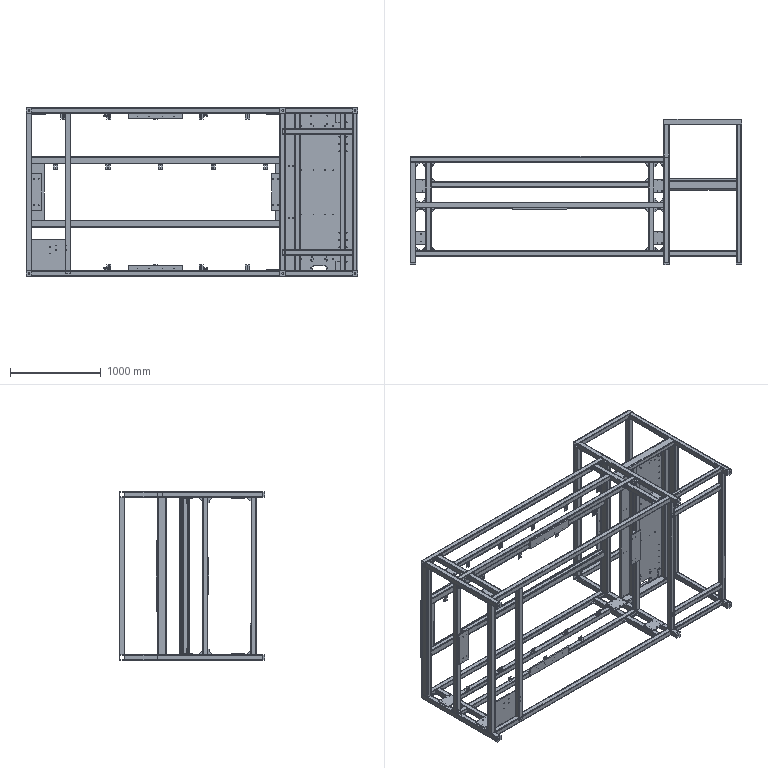Part | SolidWorks | features ReferencePattern 16, LocalLPattern 3 | 145 solids | 2615 faces | box 3660 x 1605 x 1860 mm | volume 102474394 mm3 | plane 1353 | cylinder 1219 | cone 43 | commonest cylinder face diameters 5 x368 6.4 x140 12.8 x140 6.8 x120 8.5 x99 20 x81